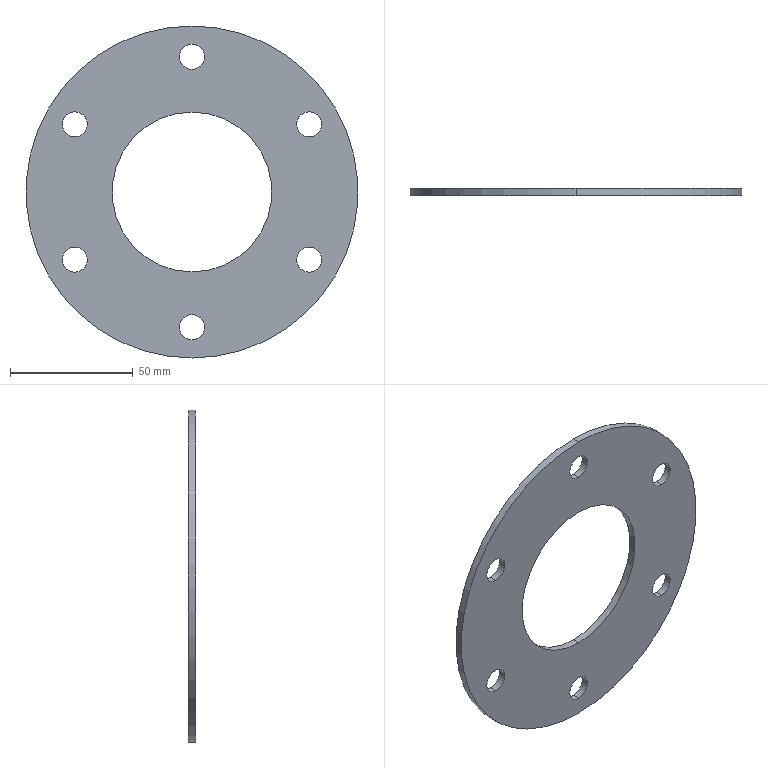Part | SolidWorks | features Extrusion 1, HoleWzd 1 | 1 solid | 18 faces | box 135 x 3 x 135 mm | volume 31516 mm3 | cylinder 16 | plane 2 | commonest cylinder face diameters 10.2 x12 65 x2 135 x2
STEP:
#1=CARTESIAN_POINT('',(0.,0.,-60.1));
#2=VERTEX_POINT('',#1);
#3=CARTESIAN_POINT('',(0.,0.,-49.9));
#4=VERTEX_POINT('',#3);
#5=CARTESIAN_POINT('',(0.,0.,-55.));
#6=DIRECTION('',(0.,1.,0.));
#7=DIRECTION('',(0.,0.,1.));
#8=AXIS2_PLACEMENT_3D('',#5,#6,#7);
#9=CIRCLE('',#8,5.1);
#10=EDGE_CURVE('',#2,#4,#9,.T.);
#11=ORIENTED_EDGE('',*,*,#10,.F.);
#12=CARTESIAN_POINT('',(0.,3.,-60.1));
#13=VERTEX_POINT('',#12);
#14=CARTESIAN_POINT('',(0.,3.,-60.1));
#15=DIRECTION('',(0.,1.,0.));
#16=VECTOR('',#15,1000.);
#17=LINE('',#14,#16);
#18=EDGE_CURVE('',#2,#13,#17,.T.);
#19=ORIENTED_EDGE('',*,*,#18,.T.);
#20=CARTESIAN_POINT('',(0.,3.,-49.9));
#21=VERTEX_POINT('',#20);
#22=CARTESIAN_POINT('',(0.,3.,-55.));
#23=DIRECTION('',(0.,1.,0.));
#24=DIRECTION('',(0.,0.,1.));
#25=AXIS2_PLACEMENT_3D('',#22,#23,#24);
#26=CIRCLE('',#25,5.1);
#27=EDGE_CURVE('',#13,#21,#26,.T.);
#28=ORIENTED_EDGE('',*,*,#27,.T.);
#29=CARTESIAN_POINT('',(0.,3.,-49.9));
#30=DIRECTION('',(0.,1.,0.));
#31=VECTOR('',#30,1000.);
#32=LINE('',#29,#31);
#33=EDGE_CURVE('',#4,#21,#32,.T.);
#34=ORIENTED_EDGE('',*,*,#33,.F.);
#35=EDGE_LOOP('',(#11,#19,#28,#34));
#36=FACE_OUTER_BOUND('',#35,.T.);
#37=CARTESIAN_POINT('',(0.,3.,-55.));
#38=DIRECTION('',(0.,1.,0.));
#39=DIRECTION('',(0.,0.,1.));
#40=AXIS2_PLACEMENT_3D('',#37,#38,#39);
#41=CYLINDRICAL_SURFACE('',#40,5.1);
#42=ADVANCED_FACE('',(#36),#41,.F.);
#43=CARTESIAN_POINT('',(-47.631,0.,-32.6));
#44=VERTEX_POINT('',#43);
#45=CARTESIAN_POINT('',(-47.631,0.,-22.4));
#46=VERTEX_POINT('',#45);
#47=CARTESIAN_POINT('',(-47.631,0.,-27.5));
#48=DIRECTION('',(0.,1.,0.));
#49=DIRECTION('',(0.,0.,1.));
#50=AXIS2_PLACEMENT_3D('',#47,#48,#49);
#51=CIRCLE('',#50,5.1);
#52=EDGE_CURVE('',#44,#46,#51,.T.);
#53=ORIENTED_EDGE('',*,*,#52,.F.);
#54=CARTESIAN_POINT('',(-47.631,3.,-32.6));
#55=VERTEX_POINT('',#54);
#56=CARTESIAN_POINT('',(-47.631,3.,-32.6));
#57=DIRECTION('',(0.,1.,0.));
#58=VECTOR('',#57,1000.);
#59=LINE('',#56,#58);
#60=EDGE_CURVE('',#44,#55,#59,.T.);
#61=ORIENTED_EDGE('',*,*,#60,.T.);
#62=CARTESIAN_POINT('',(-47.631,3.,-22.4));
#63=VERTEX_POINT('',#62);
#64=CARTESIAN_POINT('',(-47.631,3.,-27.5));
#65=DIRECTION('',(0.,1.,0.));
#66=DIRECTION('',(0.,0.,1.));
#67=AXIS2_PLACEMENT_3D('',#64,#65,#66);
#68=CIRCLE('',#67,5.1);
#69=EDGE_CURVE('',#55,#63,#68,.T.);
#70=ORIENTED_EDGE('',*,*,#69,.T.);
#71=CARTESIAN_POINT('',(-47.631,3.,-22.4));
#72=DIRECTION('',(0.,1.,0.));
#73=VECTOR('',#72,1000.);
#74=LINE('',#71,#73);
#75=EDGE_CURVE('',#46,#63,#74,.T.);
#76=ORIENTED_EDGE('',*,*,#75,.F.);
#77=EDGE_LOOP('',(#53,#61,#70,#76));
#78=FACE_OUTER_BOUND('',#77,.T.);
#79=CARTESIAN_POINT('',(-47.631,3.,-27.5));
#80=DIRECTION('',(0.,1.,0.));
#81=DIRECTION('',(0.,0.,1.));
#82=AXIS2_PLACEMENT_3D('',#79,#80,#81);
#83=CYLINDRICAL_SURFACE('',#82,5.1);
#84=ADVANCED_FACE('',(#78),#83,.F.);
#85=CARTESIAN_POINT('',(-47.631,0.,22.4));
#86=VERTEX_POINT('',#85);
#87=CARTESIAN_POINT('',(-47.631,0.,32.6));
#88=VERTEX_POINT('',#87);
#89=CARTESIAN_POINT('',(-47.631,0.,27.5));
#90=DIRECTION('',(0.,1.,0.));
#91=DIRECTION('',(0.,0.,1.));
#92=AXIS2_PLACEMENT_3D('',#89,#90,#91);
#93=CIRCLE('',#92,5.1);
#94=EDGE_CURVE('',#86,#88,#93,.T.);
#95=ORIENTED_EDGE('',*,*,#94,.F.);
#96=CARTESIAN_POINT('',(-47.631,3.,22.4));
#97=VERTEX_POINT('',#96);
#98=CARTESIAN_POINT('',(-47.631,3.,22.4));
#99=DIRECTION('',(0.,1.,0.));
#100=VECTOR('',#99,1000.);
#101=LINE('',#98,#100);
#102=EDGE_CURVE('',#86,#97,#101,.T.);
#103=ORIENTED_EDGE('',*,*,#102,.T.);
#104=CARTESIAN_POINT('',(-47.631,3.,32.6));
#105=VERTEX_POINT('',#104);
#106=CARTESIAN_POINT('',(-47.631,3.,27.5));
#107=DIRECTION('',(0.,1.,0.));
#108=DIRECTION('',(0.,0.,1.));
#109=AXIS2_PLACEMENT_3D('',#106,#107,#108);
#110=CIRCLE('',#109,5.1);
#111=EDGE_CURVE('',#97,#105,#110,.T.);
#112=ORIENTED_EDGE('',*,*,#111,.T.);
#113=CARTESIAN_POINT('',(-47.631,3.,32.6));
#114=DIRECTION('',(0.,1.,0.));
#115=VECTOR('',#114,1000.);
#116=LINE('',#113,#115);
#117=EDGE_CURVE('',#88,#105,#116,.T.);
#118=ORIENTED_EDGE('',*,*,#117,.F.);
#119=EDGE_LOOP('',(#95,#103,#112,#118));
#120=FACE_OUTER_BOUND('',#119,.T.);
#121=CARTESIAN_POINT('',(-47.631,3.,27.5));
#122=DIRECTION('',(0.,1.,0.));
#123=DIRECTION('',(0.,0.,1.));
#124=AXIS2_PLACEMENT_3D('',#121,#122,#123);
#125=CYLINDRICAL_SURFACE('',#124,5.1);
#126=ADVANCED_FACE('',(#120),#125,.F.);
#127=CARTESIAN_POINT('',(0.,0.,49.9));
#128=VERTEX_POINT('',#127);
#129=CARTESIAN_POINT('',(0.,0.,60.1));
#130=VERTEX_POINT('',#129);
#131=CARTESIAN_POINT('',(0.,0.,55.));
#132=DIRECTION('',(0.,1.,0.));
#133=DIRECTION('',(0.,0.,1.));
#134=AXIS2_PLACEMENT_3D('',#131,#132,#133);
#135=CIRCLE('',#134,5.1);
#136=EDGE_CURVE('',#128,#130,#135,.T.);
#137=ORIENTED_EDGE('',*,*,#136,.F.);
#138=CARTESIAN_POINT('',(0.,3.,49.9));
#139=VERTEX_POINT('',#138);
#140=CARTESIAN_POINT('',(0.,3.,49.9));
#141=DIRECTION('',(0.,1.,0.));
#142=VECTOR('',#141,1000.);
#143=LINE('',#140,#142);
#144=EDGE_CURVE('',#128,#139,#143,.T.);
#145=ORIENTED_EDGE('',*,*,#144,.T.);
#146=CARTESIAN_POINT('',(0.,3.,60.1));
#147=VERTEX_POINT('',#146);
#148=CARTESIAN_POINT('',(0.,3.,55.));
#149=DIRECTION('',(0.,1.,0.));
#150=DIRECTION('',(0.,0.,1.));
#151=AXIS2_PLACEMENT_3D('',#148,#149,#150);
#152=CIRCLE('',#151,5.1);
#153=EDGE_CURVE('',#139,#147,#152,.T.);
#154=ORIENTED_EDGE('',*,*,#153,.T.);
#155=CARTESIAN_POINT('',(0.,3.,60.1));
#156=DIRECTION('',(0.,1.,0.));
#157=VECTOR('',#156,1000.);
#158=LINE('',#155,#157);
#159=EDGE_CURVE('',#130,#147,#158,.T.);
#160=ORIENTED_EDGE('',*,*,#159,.F.);
#161=EDGE_LOOP('',(#137,#145,#154,#160));
#162=FACE_OUTER_BOUND('',#161,.T.);
#163=CARTESIAN_POINT('',(0.,3.,55.));
#164=DIRECTION('',(0.,1.,0.));
#165=DIRECTION('',(0.,0.,1.));
#166=AXIS2_PLACEMENT_3D('',#163,#164,#165);
#167=CYLINDRICAL_SURFACE('',#166,5.1);
#168=ADVANCED_FACE('',(#162),#167,.F.);
#169=CARTESIAN_POINT('',(47.631,0.,22.4));
#170=VERTEX_POINT('',#169);
#171=CARTESIAN_POINT('',(47.631,0.,32.6));
#172=VERTEX_POINT('',#171);
#173=CARTESIAN_POINT('',(47.631,0.,27.5));
#174=DIRECTION('',(0.,1.,0.));
#175=DIRECTION('',(0.,0.,1.));
#176=AXIS2_PLACEMENT_3D('',#173,#174,#175);
#177=CIRCLE('',#176,5.1);
#178=EDGE_CURVE('',#170,#172,#177,.T.);
#179=ORIENTED_EDGE('',*,*,#178,.F.);
#180=CARTESIAN_POINT('',(47.631,3.,22.4));
#181=VERTEX_POINT('',#180);
#182=CARTESIAN_POINT('',(47.631,3.,22.4));
#183=DIRECTION('',(0.,1.,0.));
#184=VECTOR('',#183,1000.);
#185=LINE('',#182,#184);
#186=EDGE_CURVE('',#170,#181,#185,.T.);
#187=ORIENTED_EDGE('',*,*,#186,.T.);
#188=CARTESIAN_POINT('',(47.631,3.,32.6));
#189=VERTEX_POINT('',#188);
#190=CARTESIAN_POINT('',(47.631,3.,27.5));
#191=DIRECTION('',(0.,1.,0.));
#192=DIRECTION('',(0.,0.,1.));
#193=AXIS2_PLACEMENT_3D('',#190,#191,#192);
#194=CIRCLE('',#193,5.1);
#195=EDGE_CURVE('',#181,#189,#194,.T.);
#196=ORIENTED_EDGE('',*,*,#195,.T.);
#197=CARTESIAN_POINT('',(47.631,3.,32.6));
#198=DIRECTION('',(0.,1.,0.));
#199=VECTOR('',#198,1000.);
#200=LINE('',#197,#199);
#201=EDGE_CURVE('',#172,#189,#200,.T.);
#202=ORIENTED_EDGE('',*,*,#201,.F.);
#203=EDGE_LOOP('',(#179,#187,#196,#202));
#204=FACE_OUTER_BOUND('',#203,.T.);
#205=CARTESIAN_POINT('',(47.631,3.,27.5));
#206=DIRECTION('',(0.,1.,0.));
#207=DIRECTION('',(0.,0.,1.));
#208=AXIS2_PLACEMENT_3D('',#205,#206,#207);
#209=CYLINDRICAL_SURFACE('',#208,5.1);
#210=ADVANCED_FACE('',(#204),#209,.F.);
#211=CARTESIAN_POINT('',(47.631,0.,-32.6));
#212=VERTEX_POINT('',#211);
#213=CARTESIAN_POINT('',(47.631,0.,-22.4));
#214=VERTEX_POINT('',#213);
#215=CARTESIAN_POINT('',(47.631,0.,-27.5));
#216=DIRECTION('',(0.,1.,0.));
#217=DIRECTION('',(0.,0.,1.));
#218=AXIS2_PLACEMENT_3D('',#215,#216,#217);
#219=CIRCLE('',#218,5.1);
#220=EDGE_CURVE('',#212,#214,#219,.T.);
#221=ORIENTED_EDGE('',*,*,#220,.F.);
#222=CARTESIAN_POINT('',(47.631,3.,-32.6));
#223=VERTEX_POINT('',#222);
#224=CARTESIAN_POINT('',(47.631,3.,-32.6));
#225=DIRECTION('',(0.,1.,0.));
#226=VECTOR('',#225,1000.);
#227=LINE('',#224,#226);
#228=EDGE_CURVE('',#212,#223,#227,.T.);
#229=ORIENTED_EDGE('',*,*,#228,.T.);
#230=CARTESIAN_POINT('',(47.631,3.,-22.4));
#231=VERTEX_POINT('',#230);
#232=CARTESIAN_POINT('',(47.631,3.,-27.5));
#233=DIRECTION('',(0.,1.,0.));
#234=DIRECTION('',(0.,0.,1.));
#235=AXIS2_PLACEMENT_3D('',#232,#233,#234);
#236=CIRCLE('',#235,5.1);
#237=EDGE_CURVE('',#223,#231,#236,.T.);
#238=ORIENTED_EDGE('',*,*,#237,.T.);
#239=CARTESIAN_POINT('',(47.631,3.,-22.4));
#240=DIRECTION('',(0.,1.,0.));
#241=VECTOR('',#240,1000.);
#242=LINE('',#239,#241);
#243=EDGE_CURVE('',#214,#231,#242,.T.);
#244=ORIENTED_EDGE('',*,*,#243,.F.);
#245=EDGE_LOOP('',(#221,#229,#238,#244));
#246=FACE_OUTER_BOUND('',#245,.T.);
#247=CARTESIAN_POINT('',(47.631,3.,-27.5));
#248=DIRECTION('',(0.,1.,0.));
#249=DIRECTION('',(0.,0.,1.));
#250=AXIS2_PLACEMENT_3D('',#247,#248,#249);
#251=CYLINDRICAL_SURFACE('',#250,5.1);
#252=ADVANCED_FACE('',(#246),#251,.F.);
#253=CARTESIAN_POINT('',(0.,3.,-32.5));
#254=VERTEX_POINT('',#253);
#255=CARTESIAN_POINT('',(0.,3.,32.5));
#256=VERTEX_POINT('',#255);
#257=CARTESIAN_POINT('',(0.,3.,0.));
#258=DIRECTION('',(0.,1.,0.));
#259=DIRECTION('',(0.,0.,1.));
#260=AXIS2_PLACEMENT_3D('',#257,#258,#259);
#261=CIRCLE('',#260,32.5);
#262=EDGE_CURVE('',#254,#256,#261,.T.);
#263=ORIENTED_EDGE('',*,*,#262,.T.);
#264=CARTESIAN_POINT('',(0.,0.,32.5));
#265=VERTEX_POINT('',#264);
#266=CARTESIAN_POINT('',(0.,3.,32.5));
#267=DIRECTION('',(0.,-1.,0.));
#268=VECTOR('',#267,1000.);
#269=LINE('',#266,#268);
#270=EDGE_CURVE('',#256,#265,#269,.T.);
#271=ORIENTED_EDGE('',*,*,#270,.T.);
#272=CARTESIAN_POINT('',(0.,0.,-32.5));
#273=VERTEX_POINT('',#272);
#274=CARTESIAN_POINT('',(0.,0.,0.));
#275=DIRECTION('',(0.,1.,0.));
#276=DIRECTION('',(0.,0.,1.));
#277=AXIS2_PLACEMENT_3D('',#274,#275,#276);
#278=CIRCLE('',#277,32.5);
#279=EDGE_CURVE('',#273,#265,#278,.T.);
#280=ORIENTED_EDGE('',*,*,#279,.F.);
#281=CARTESIAN_POINT('',(0.,3.,-32.5));
#282=DIRECTION('',(0.,-1.,0.));
#283=VECTOR('',#282,1000.);
#284=LINE('',#281,#283);
#285=EDGE_CURVE('',#254,#273,#284,.T.);
#286=ORIENTED_EDGE('',*,*,#285,.F.);
#287=EDGE_LOOP('',(#263,#271,#280,#286));
#288=FACE_OUTER_BOUND('',#287,.T.);
#289=CARTESIAN_POINT('',(0.,3.,0.));
#290=DIRECTION('',(0.,-1.,0.));
#291=DIRECTION('',(0.,0.,-1.));
#292=AXIS2_PLACEMENT_3D('',#289,#290,#291);
#293=CYLINDRICAL_SURFACE('',#292,32.5);
#294=ADVANCED_FACE('',(#288),#293,.F.);
#295=CARTESIAN_POINT('',(0.,3.,67.5));
#296=VERTEX_POINT('',#295);
#297=CARTESIAN_POINT('',(0.,3.,-67.5));
#298=VERTEX_POINT('',#297);
#299=CARTESIAN_POINT('',(0.,3.,0.));
#300=DIRECTION('',(0.,1.,0.));
#301=DIRECTION('',(0.,0.,1.));
#302=AXIS2_PLACEMENT_3D('',#299,#300,#301);
#303=CIRCLE('',#302,67.5);
#304=EDGE_CURVE('',#296,#298,#303,.T.);
#305=ORIENTED_EDGE('',*,*,#304,.F.);
#306=CARTESIAN_POINT('',(0.,0.,67.5));
#307=VERTEX_POINT('',#306);
#308=CARTESIAN_POINT('',(0.,3.,67.5));
#309=DIRECTION('',(0.,-1.,0.));
#310=VECTOR('',#309,1000.);
#311=LINE('',#308,#310);
#312=EDGE_CURVE('',#296,#307,#311,.T.);
#313=ORIENTED_EDGE('',*,*,#312,.T.);
#314=CARTESIAN_POINT('',(0.,0.,-67.5));
#315=VERTEX_POINT('',#314);
#316=CARTESIAN_POINT('',(0.,0.,0.));
#317=DIRECTION('',(0.,1.,0.));
#318=DIRECTION('',(0.,0.,1.));
#319=AXIS2_PLACEMENT_3D('',#316,#317,#318);
#320=CIRCLE('',#319,67.5);
#321=EDGE_CURVE('',#307,#315,#320,.T.);
#322=ORIENTED_EDGE('',*,*,#321,.T.);
#323=CARTESIAN_POINT('',(0.,3.,-67.5));
#324=DIRECTION('',(0.,-1.,0.));
#325=VECTOR('',#324,1000.);
#326=LINE('',#323,#325);
#327=EDGE_CURVE('',#298,#315,#326,.T.);
#328=ORIENTED_EDGE('',*,*,#327,.F.);
#329=EDGE_LOOP('',(#305,#313,#322,#328));
#330=FACE_OUTER_BOUND('',#329,.T.);
#331=CARTESIAN_POINT('',(0.,3.,0.));
#332=DIRECTION('',(0.,-1.,0.));
#333=DIRECTION('',(0.,0.,-1.));
#334=AXIS2_PLACEMENT_3D('',#331,#332,#333);
#335=CYLINDRICAL_SURFACE('',#334,67.5);
#336=ADVANCED_FACE('',(#330),#335,.T.);
#337=CARTESIAN_POINT('',(0.,3.,-55.));
#338=DIRECTION('',(0.,1.,0.));
#339=DIRECTION('',(0.,0.,1.));
#340=AXIS2_PLACEMENT_3D('',#337,#338,#339);
#341=CIRCLE('',#340,5.1);
#342=EDGE_CURVE('',#21,#13,#341,.T.);
#343=ORIENTED_EDGE('',*,*,#342,.F.);
#344=ORIENTED_EDGE('',*,*,#27,.F.);
#345=EDGE_LOOP('',(#343,#344));
#346=FACE_BOUND('',#345,.T.);
#347=CARTESIAN_POINT('',(-47.631,3.,-27.5));
#348=DIRECTION('',(0.,1.,0.));
#349=DIRECTION('',(0.,0.,1.));
#350=AXIS2_PLACEMENT_3D('',#347,#348,#349);
#351=CIRCLE('',#350,5.1);
#352=EDGE_CURVE('',#63,#55,#351,.T.);
#353=ORIENTED_EDGE('',*,*,#352,.F.);
#354=ORIENTED_EDGE('',*,*,#69,.F.);
#355=EDGE_LOOP('',(#353,#354));
#356=FACE_BOUND('',#355,.T.);
#357=CARTESIAN_POINT('',(-47.631,3.,27.5));
#358=DIRECTION('',(0.,1.,0.));
#359=DIRECTION('',(0.,0.,1.));
#360=AXIS2_PLACEMENT_3D('',#357,#358,#359);
#361=CIRCLE('',#360,5.1);
#362=EDGE_CURVE('',#105,#97,#361,.T.);
#363=ORIENTED_EDGE('',*,*,#362,.F.);
#364=ORIENTED_EDGE('',*,*,#111,.F.);
#365=EDGE_LOOP('',(#363,#364));
#366=FACE_BOUND('',#365,.T.);
#367=CARTESIAN_POINT('',(0.,3.,55.));
#368=DIRECTION('',(0.,1.,0.));
#369=DIRECTION('',(0.,0.,1.));
#370=AXIS2_PLACEMENT_3D('',#367,#368,#369);
#371=CIRCLE('',#370,5.1);
#372=EDGE_CURVE('',#147,#139,#371,.T.);
#373=ORIENTED_EDGE('',*,*,#372,.F.);
#374=ORIENTED_EDGE('',*,*,#153,.F.);
#375=EDGE_LOOP('',(#373,#374));
#376=FACE_BOUND('',#375,.T.);
#377=CARTESIAN_POINT('',(47.631,3.,27.5));
#378=DIRECTION('',(0.,1.,0.));
#379=DIRECTION('',(0.,0.,1.));
#380=AXIS2_PLACEMENT_3D('',#377,#378,#379);
#381=CIRCLE('',#380,5.1);
#382=EDGE_CURVE('',#189,#181,#381,.T.);
#383=ORIENTED_EDGE('',*,*,#382,.F.);
#384=ORIENTED_EDGE('',*,*,#195,.F.);
#385=EDGE_LOOP('',(#383,#384));
#386=FACE_BOUND('',#385,.T.);
#387=CARTESIAN_POINT('',(47.631,3.,-27.5));
#388=DIRECTION('',(0.,1.,0.));
#389=DIRECTION('',(0.,0.,1.));
#390=AXIS2_PLACEMENT_3D('',#387,#388,#389);
#391=CIRCLE('',#390,5.1);
#392=EDGE_CURVE('',#231,#223,#391,.T.);
#393=ORIENTED_EDGE('',*,*,#392,.F.);
#394=ORIENTED_EDGE('',*,*,#237,.F.);
#395=EDGE_LOOP('',(#393,#394));
#396=FACE_BOUND('',#395,.T.);
#397=CARTESIAN_POINT('',(0.,3.,0.));
#398=DIRECTION('',(0.,1.,0.));
#399=DIRECTION('',(0.,0.,1.));
#400=AXIS2_PLACEMENT_3D('',#397,#398,#399);
#401=CIRCLE('',#400,67.5);
#402=EDGE_CURVE('',#298,#296,#401,.T.);
#403=ORIENTED_EDGE('',*,*,#402,.T.);
#404=ORIENTED_EDGE('',*,*,#304,.T.);
#405=EDGE_LOOP('',(#403,#404));
#406=FACE_OUTER_BOUND('',#405,.T.);
#407=ORIENTED_EDGE('',*,*,#262,.F.);
#408=CARTESIAN_POINT('',(0.,3.,0.));
#409=DIRECTION('',(0.,1.,0.));
#410=DIRECTION('',(0.,0.,1.));
#411=AXIS2_PLACEMENT_3D('',#408,#409,#410);
#412=CIRCLE('',#411,32.5);
#413=EDGE_CURVE('',#256,#254,#412,.T.);
#414=ORIENTED_EDGE('',*,*,#413,.F.);
#415=EDGE_LOOP('',(#407,#414));
#416=FACE_BOUND('',#415,.T.);
#417=CARTESIAN_POINT('',(0.,3.,0.));
#418=DIRECTION('',(0.,1.,0.));
#419=DIRECTION('',(0.,0.,1.));
#420=AXIS2_PLACEMENT_3D('',#417,#418,#419);
#421=PLANE('',#420);
#422=ADVANCED_FACE('',(#346,#356,#366,#376,#386,#396,#406,#416),#421,.T.);
#423=CARTESIAN_POINT('',(0.,0.,-55.));
#424=DIRECTION('',(0.,1.,0.));
#425=DIRECTION('',(0.,0.,1.));
#426=AXIS2_PLACEMENT_3D('',#423,#424,#425);
#427=CIRCLE('',#426,5.1);
#428=EDGE_CURVE('',#4,#2,#427,.T.);
#429=ORIENTED_EDGE('',*,*,#428,.T.);
#430=ORIENTED_EDGE('',*,*,#10,.T.);
#431=EDGE_LOOP('',(#429,#430));
#432=FACE_BOUND('',#431,.T.);
#433=CARTESIAN_POINT('',(-47.631,0.,-27.5));
#434=DIRECTION('',(0.,1.,0.));
#435=DIRECTION('',(0.,0.,1.));
#436=AXIS2_PLACEMENT_3D('',#433,#434,#435);
#437=CIRCLE('',#436,5.1);
#438=EDGE_CURVE('',#46,#44,#437,.T.);
#439=ORIENTED_EDGE('',*,*,#438,.T.);
#440=ORIENTED_EDGE('',*,*,#52,.T.);
#441=EDGE_LOOP('',(#439,#440));
#442=FACE_BOUND('',#441,.T.);
#443=CARTESIAN_POINT('',(-47.631,0.,27.5));
#444=DIRECTION('',(0.,1.,0.));
#445=DIRECTION('',(0.,0.,1.));
#446=AXIS2_PLACEMENT_3D('',#443,#444,#445);
#447=CIRCLE('',#446,5.1);
#448=EDGE_CURVE('',#88,#86,#447,.T.);
#449=ORIENTED_EDGE('',*,*,#448,.T.);
#450=ORIENTED_EDGE('',*,*,#94,.T.);
#451=EDGE_LOOP('',(#449,#450));
#452=FACE_BOUND('',#451,.T.);
#453=CARTESIAN_POINT('',(0.,0.,55.));
#454=DIRECTION('',(0.,1.,0.));
#455=DIRECTION('',(0.,0.,1.));
#456=AXIS2_PLACEMENT_3D('',#453,#454,#455);
#457=CIRCLE('',#456,5.1);
#458=EDGE_CURVE('',#130,#128,#457,.T.);
#459=ORIENTED_EDGE('',*,*,#458,.T.);
#460=ORIENTED_EDGE('',*,*,#136,.T.);
#461=EDGE_LOOP('',(#459,#460));
#462=FACE_BOUND('',#461,.T.);
#463=CARTESIAN_POINT('',(47.631,0.,27.5));
#464=DIRECTION('',(0.,1.,0.));
#465=DIRECTION('',(0.,0.,1.));
#466=AXIS2_PLACEMENT_3D('',#463,#464,#465);
#467=CIRCLE('',#466,5.1);
#468=EDGE_CURVE('',#172,#170,#467,.T.);
#469=ORIENTED_EDGE('',*,*,#468,.T.);
#470=ORIENTED_EDGE('',*,*,#178,.T.);
#471=EDGE_LOOP('',(#469,#470));
#472=FACE_BOUND('',#471,.T.);
#473=CARTESIAN_POINT('',(47.631,0.,-27.5));
#474=DIRECTION('',(0.,1.,0.));
#475=DIRECTION('',(0.,0.,1.));
#476=AXIS2_PLACEMENT_3D('',#473,#474,#475);
#477=CIRCLE('',#476,5.1);
#478=EDGE_CURVE('',#214,#212,#477,.T.);
#479=ORIENTED_EDGE('',*,*,#478,.T.);
#480=ORIENTED_EDGE('',*,*,#220,.T.);
#481=EDGE_LOOP('',(#479,#480));
#482=FACE_BOUND('',#481,.T.);
#483=CARTESIAN_POINT('',(0.,0.,0.));
#484=DIRECTION('',(0.,1.,0.));
#485=DIRECTION('',(0.,0.,1.));
#486=AXIS2_PLACEMENT_3D('',#483,#484,#485);
#487=CIRCLE('',#486,67.5);
#488=EDGE_CURVE('',#315,#307,#487,.T.);
#489=ORIENTED_EDGE('',*,*,#488,.F.);
#490=ORIENTED_EDGE('',*,*,#321,.F.);
#491=EDGE_LOOP('',(#489,#490));
#492=FACE_OUTER_BOUND('',#491,.T.);
#493=ORIENTED_EDGE('',*,*,#279,.T.);
#494=CARTESIAN_POINT('',(0.,0.,0.));
#495=DIRECTION('',(0.,1.,0.));
#496=DIRECTION('',(0.,0.,1.));
#497=AXIS2_PLACEMENT_3D('',#494,#495,#496);
#498=CIRCLE('',#497,32.5);
#499=EDGE_CURVE('',#265,#273,#498,.T.);
#500=ORIENTED_EDGE('',*,*,#499,.T.);
#501=EDGE_LOOP('',(#493,#500));
#502=FACE_BOUND('',#501,.T.);
#503=CARTESIAN_POINT('',(0.,0.,0.));
#504=DIRECTION('',(0.,1.,0.));
#505=DIRECTION('',(0.,0.,1.));
#506=AXIS2_PLACEMENT_3D('',#503,#504,#505);
#507=PLANE('',#506);
#508=ADVANCED_FACE('',(#432,#442,#452,#462,#472,#482,#492,#502),#507,.F.);
#509=ORIENTED_EDGE('',*,*,#312,.F.);
#510=ORIENTED_EDGE('',*,*,#402,.F.);
#511=ORIENTED_EDGE('',*,*,#327,.T.);
#512=ORIENTED_EDGE('',*,*,#488,.T.);
#513=EDGE_LOOP('',(#509,#510,#511,#512));
#514=FACE_OUTER_BOUND('',#513,.T.);
#515=CARTESIAN_POINT('',(0.,3.,0.));
#516=DIRECTION('',(0.,-1.,0.));
#517=DIRECTION('',(0.,0.,-1.));
#518=AXIS2_PLACEMENT_3D('',#515,#516,#517);
#519=CYLINDRICAL_SURFACE('',#518,67.5);
#520=ADVANCED_FACE('',(#514),#519,.T.);
#521=ORIENTED_EDGE('',*,*,#270,.F.);
#522=ORIENTED_EDGE('',*,*,#413,.T.);
#523=ORIENTED_EDGE('',*,*,#285,.T.);
#524=ORIENTED_EDGE('',*,*,#499,.F.);
#525=EDGE_LOOP('',(#521,#522,#523,#524));
#526=FACE_OUTER_BOUND('',#525,.T.);
#527=CARTESIAN_POINT('',(0.,3.,0.));
#528=DIRECTION('',(0.,-1.,0.));
#529=DIRECTION('',(0.,0.,-1.));
#530=AXIS2_PLACEMENT_3D('',#527,#528,#529);
#531=CYLINDRICAL_SURFACE('',#530,32.5);
#532=ADVANCED_FACE('',(#526),#531,.F.);
#533=ORIENTED_EDGE('',*,*,#228,.F.);
#534=ORIENTED_EDGE('',*,*,#478,.F.);
#535=ORIENTED_EDGE('',*,*,#243,.T.);
#536=ORIENTED_EDGE('',*,*,#392,.T.);
#537=EDGE_LOOP('',(#533,#534,#535,#536));
#538=FACE_OUTER_BOUND('',#537,.T.);
#539=CARTESIAN_POINT('',(47.631,3.,-27.5));
#540=DIRECTION('',(0.,1.,0.));
#541=DIRECTION('',(0.,0.,1.));
#542=AXIS2_PLACEMENT_3D('',#539,#540,#541);
#543=CYLINDRICAL_SURFACE('',#542,5.1);
#544=ADVANCED_FACE('',(#538),#543,.F.);
#545=ORIENTED_EDGE('',*,*,#186,.F.);
#546=ORIENTED_EDGE('',*,*,#468,.F.);
#547=ORIENTED_EDGE('',*,*,#201,.T.);
#548=ORIENTED_EDGE('',*,*,#382,.T.);
#549=EDGE_LOOP('',(#545,#546,#547,#548));
#550=FACE_OUTER_BOUND('',#549,.T.);
#551=CARTESIAN_POINT('',(47.631,3.,27.5));
#552=DIRECTION('',(0.,1.,0.));
#553=DIRECTION('',(0.,0.,1.));
#554=AXIS2_PLACEMENT_3D('',#551,#552,#553);
#555=CYLINDRICAL_SURFACE('',#554,5.1);
#556=ADVANCED_FACE('',(#550),#555,.F.);
#557=ORIENTED_EDGE('',*,*,#144,.F.);
#558=ORIENTED_EDGE('',*,*,#458,.F.);
#559=ORIENTED_EDGE('',*,*,#159,.T.);
#560=ORIENTED_EDGE('',*,*,#372,.T.);
#561=EDGE_LOOP('',(#557,#558,#559,#560));
#562=FACE_OUTER_BOUND('',#561,.T.);
#563=CARTESIAN_POINT('',(0.,3.,55.));
#564=DIRECTION('',(0.,1.,0.));
#565=DIRECTION('',(0.,0.,1.));
#566=AXIS2_PLACEMENT_3D('',#563,#564,#565);
#567=CYLINDRICAL_SURFACE('',#566,5.1);
#568=ADVANCED_FACE('',(#562),#567,.F.);
#569=ORIENTED_EDGE('',*,*,#102,.F.);
#570=ORIENTED_EDGE('',*,*,#448,.F.);
#571=ORIENTED_EDGE('',*,*,#117,.T.);
#572=ORIENTED_EDGE('',*,*,#362,.T.);
#573=EDGE_LOOP('',(#569,#570,#571,#572));
#574=FACE_OUTER_BOUND('',#573,.T.);
#575=CARTESIAN_POINT('',(-47.631,3.,27.5));
#576=DIRECTION('',(0.,1.,0.));
#577=DIRECTION('',(0.,0.,1.));
#578=AXIS2_PLACEMENT_3D('',#575,#576,#577);
#579=CYLINDRICAL_SURFACE('',#578,5.1);
#580=ADVANCED_FACE('',(#574),#579,.F.);
#581=ORIENTED_EDGE('',*,*,#60,.F.);
#582=ORIENTED_EDGE('',*,*,#438,.F.);
#583=ORIENTED_EDGE('',*,*,#75,.T.);
#584=ORIENTED_EDGE('',*,*,#352,.T.);
#585=EDGE_LOOP('',(#581,#582,#583,#584));
#586=FACE_OUTER_BOUND('',#585,.T.);
#587=CARTESIAN_POINT('',(-47.631,3.,-27.5));
#588=DIRECTION('',(0.,1.,0.));
#589=DIRECTION('',(0.,0.,1.));
#590=AXIS2_PLACEMENT_3D('',#587,#588,#589);
#591=CYLINDRICAL_SURFACE('',#590,5.1);
#592=ADVANCED_FACE('',(#586),#591,.F.);
#593=ORIENTED_EDGE('',*,*,#18,.F.);
#594=ORIENTED_EDGE('',*,*,#428,.F.);
#595=ORIENTED_EDGE('',*,*,#33,.T.);
#596=ORIENTED_EDGE('',*,*,#342,.T.);
#597=EDGE_LOOP('',(#593,#594,#595,#596));
#598=FACE_OUTER_BOUND('',#597,.T.);
#599=CARTESIAN_POINT('',(0.,3.,-55.));
#600=DIRECTION('',(0.,1.,0.));
#601=DIRECTION('',(0.,0.,1.));
#602=AXIS2_PLACEMENT_3D('',#599,#600,#601);
#603=CYLINDRICAL_SURFACE('',#602,5.1);
#604=ADVANCED_FACE('',(#598),#603,.F.);
#605=CLOSED_SHELL('',(#42,#84,#126,#168,#210,#252,#294,#336,#422,#508,#520,#532,#544,#556,#568,#580,#592,#604));
#606=MANIFOLD_SOLID_BREP('',#605);
#607=CARTESIAN_POINT('',(0.,0.,0.));
#608=DIRECTION('',(0.,0.,1.));
#609=DIRECTION('',(1.,0.,0.));
#610=AXIS2_PLACEMENT_3D('',#607,#608,#609);
#611=(LENGTH_UNIT()NAMED_UNIT(*)SI_UNIT(.MILLI.,.METRE.));
#612=UNCERTAINTY_MEASURE_WITH_UNIT(LENGTH_MEASURE(0.00001),#611,'','');
#613=(NAMED_UNIT(*)PLANE_ANGLE_UNIT()SI_UNIT($,.RADIAN.));
#614=(NAMED_UNIT(*)SI_UNIT($,.STERADIAN.)SOLID_ANGLE_UNIT());
#615=(GEOMETRIC_REPRESENTATION_CONTEXT(3)GLOBAL_UNCERTAINTY_ASSIGNED_CONTEXT((#612))GLOBAL_UNIT_ASSIGNED_CONTEXT((#611,#613,#614))REPRESENTATION_CONTEXT('',''));
#616=ADVANCED_BREP_SHAPE_REPRESENTATION('',(#606,#610),#615);